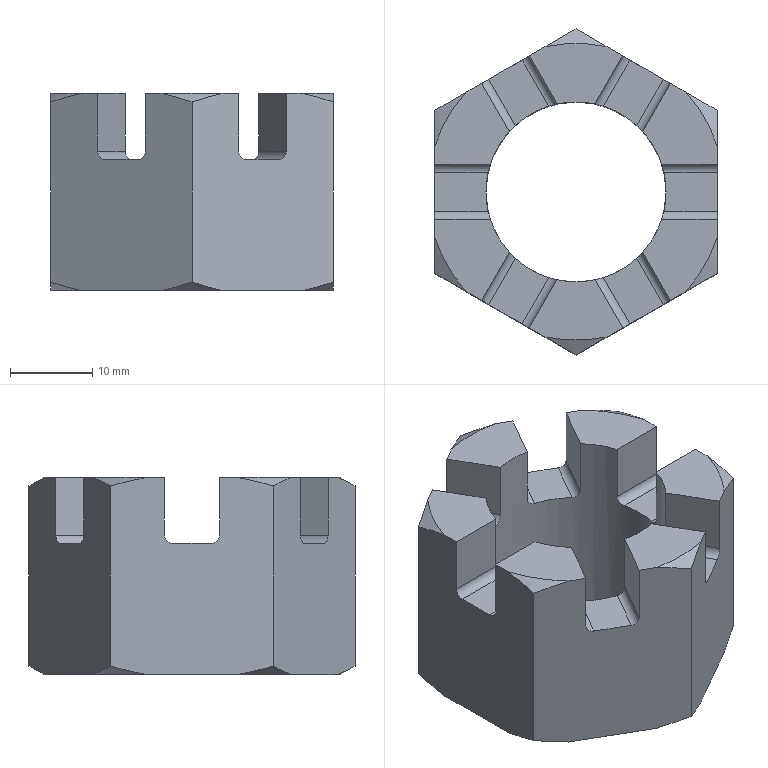Part | SolidWorks | features Cut 3, Chamfer 1, CirPattern 1, Extrusion 1 | 1 solid | 59 faces | box 34.251 x 39.55 x 23.9 mm | volume 13268 mm3 | plane 31 | cone 14 | cylinder 14 | commonest cylinder face diameters 2 x12 21.835 x2